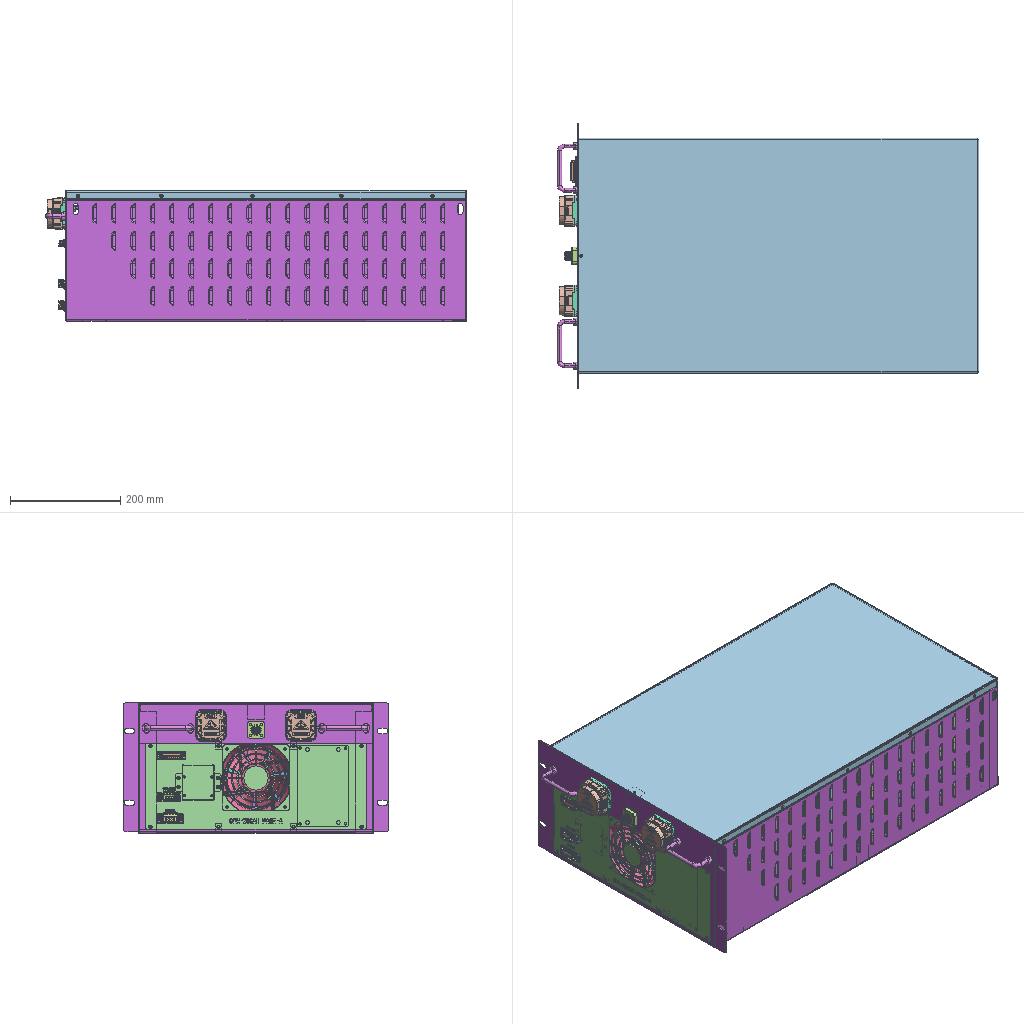Assembly | NX | 135 different items | 178 placed | box 763 x 481 x 237 mm
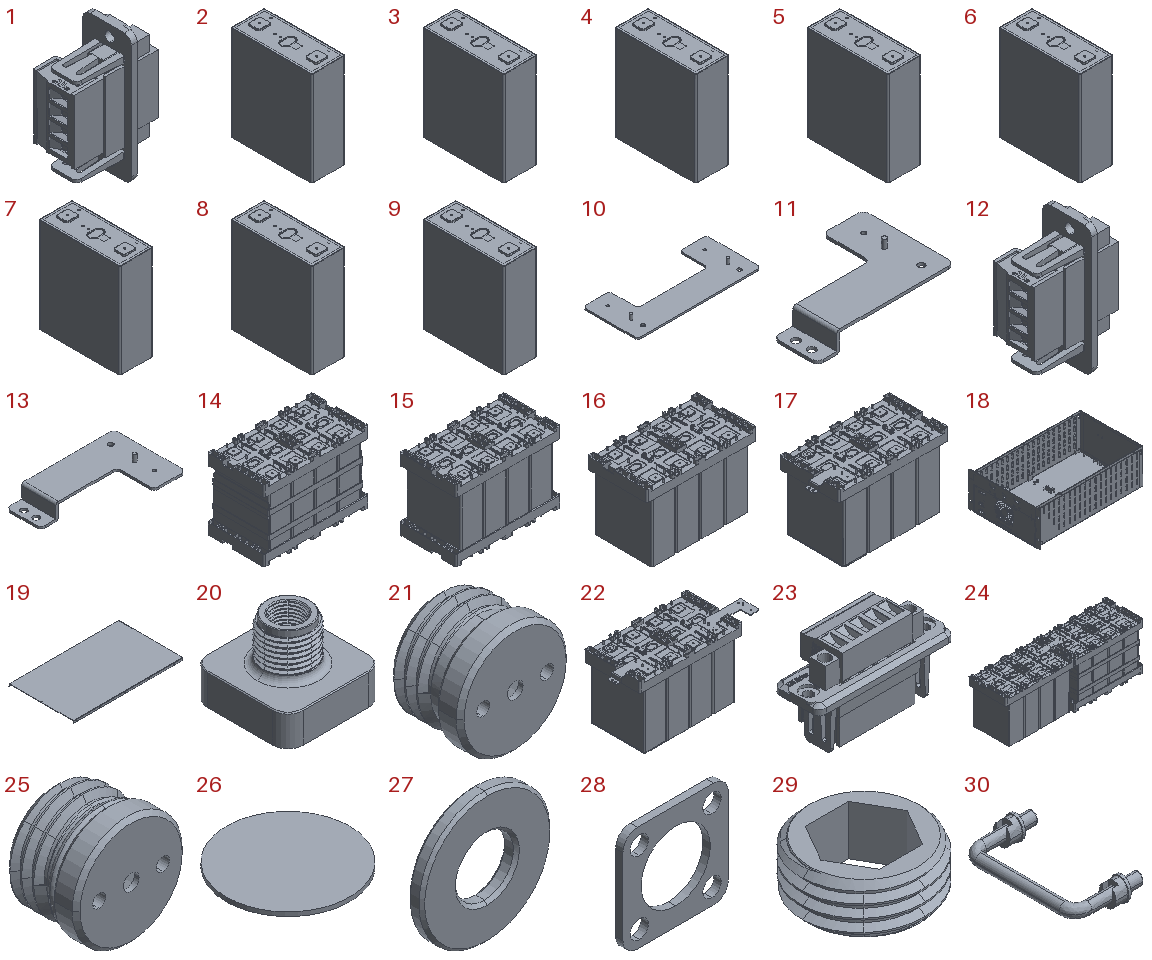Parts list (item | quantity | parent item | size | volume | features):
1 | x1 | - | - | 9257 mm3 | features BREP 21
2 | x1 | in 17 | 71.65 x 173.93 x 207.23 mm | 2540512 mm3 | features BREP 1
3 | x1 | in 16 | 71.65 x 173.93 x 207.23 mm | 2540512 mm3 | features BREP 1
4 | x1 | in 17 | 71.65 x 173.93 x 207.23 mm | 2540512 mm3 | features BREP 1
5 | x1 | in 16 | 71.65 x 173.93 x 207.23 mm | 2540523 mm3 | features BREP 2
6 | x1 | in 17 | 71.65 x 173.93 x 207.23 mm | 2540512 mm3 | features BREP 1
7 | x1 | - | 71.65 x 173.93 x 207.23 mm | 2540512 mm3 | features BREP 1
8 | x1 | - | 71.65 x 173.93 x 207.23 mm | 2540512 mm3 | features BREP 1
9 | x1 | in 14 | 71.65 x 173.93 x 207.23 mm | 2540523 mm3 | features BREP 2
10 | x2 | in 22, 24 | 142 x 62.9 x 8 mm | 12580 mm3 | features BREP 1
11 | x1 | - | 95.45 x 63.5 x 20.5 mm | 8247 mm3 | features BREP 1
12 | x1 | in 70 | - | 9257 mm3 | features BREP 21
13 | x1 | in 17 | 95.45 x 63.5 x 20.5 mm | 8247 mm3 | features BREP 1
14 | x1 | in 24 | 333 x 182 x 228.75 mm | 10791540 mm3 | features BREP 4
15 | x1 | - | 333 x 182 x 227.965 mm | 10643125 mm3 | features BREP 10
16 | x1 | in 24 | 333 x 182 x 217.08 mm | 10398899 mm3 | features BREP 11
17 | x1 | in 22 | 360 x 182 x 216.365 mm | 10554329 mm3 | features BREP 20
18 | x1 | in 38 | - | 1890874 mm3 | features BREP 3
19 | x1 | in 70 | 724.237 x 425.821 x 15 mm | 661919 mm3 | features BREP 1
20 | x1 | in 39 | 31 x 31 x 24 mm | 8742 mm3 | features BREP 1
21 | x1 | in 25 | 13.8 x 9.7 x 13.8 mm | 672.716 mm3 | features BREP 1
22 | x1 | in 94 | 431.925 x 182 x 216.365 mm | 10566909 mm3 | features BREP 21
23 | x1 | - | - | 11022 mm3 | features BREP 24
24 | x1 | in 94 | - | 21203019 mm3 | features BREP 27
25 | x1 | in 39 | 13.8 x 9.7 x 13.8 mm | 702.321 mm3 | features BREP 2
26 | x1 | in 39 | 9 x 9 x 0.3 mm | 19.085 mm3 | features BREP 1
27 | x2 | in 39 | 9 x 1 x 9 mm | 49.417 mm3 | features BREP 1
28 | x1 | in 39 | 29 x 2 x 29 mm | 930.394 mm3 | features BREP 1
29 | x1 | in 39 | 9.9 x 9.9 x 4 mm | 143.224 mm3 | features BREP 1
30 | x2 | in 70 | 51.75 x 94.4 x 18 mm | 11603 mm3 | features BREP 1
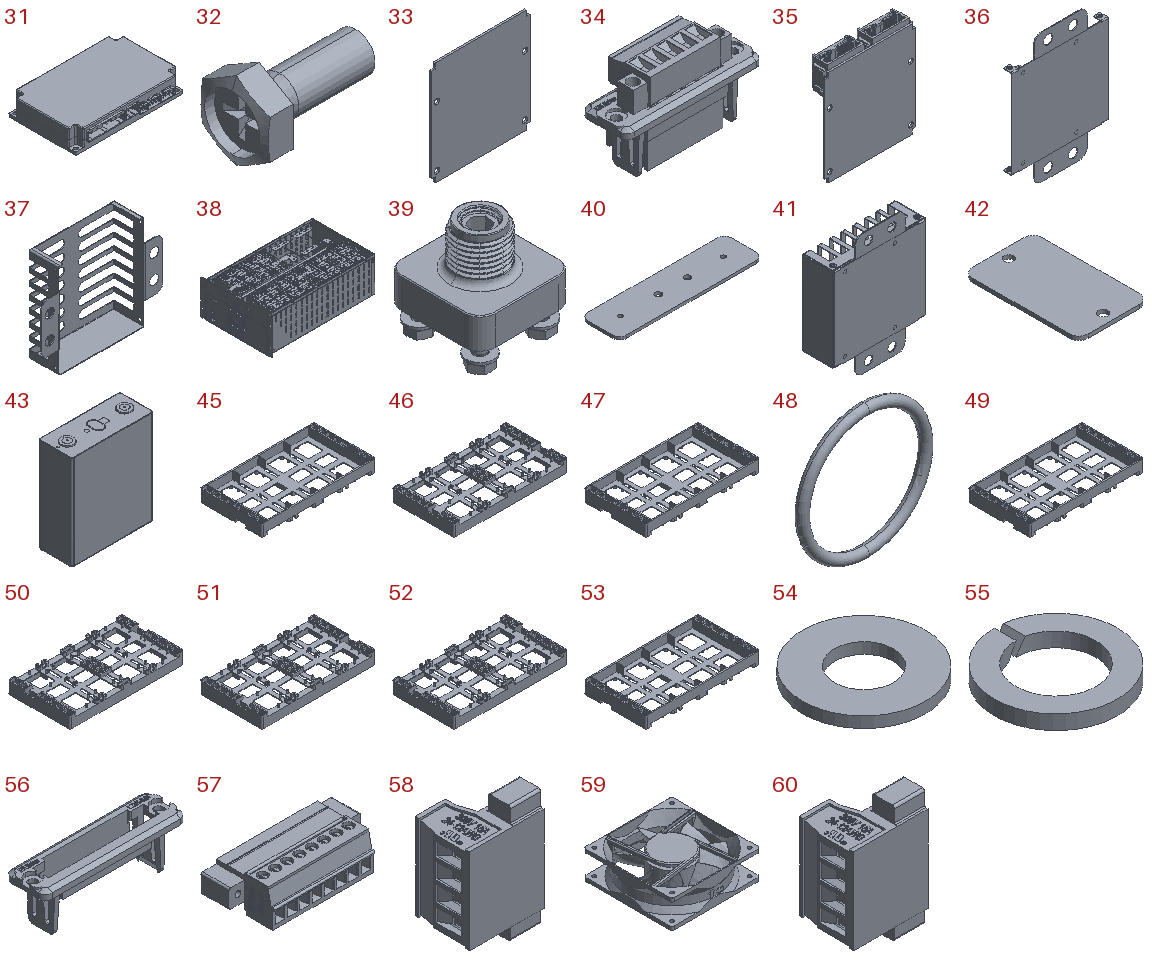31 | x1 | - | 146 x 94 x 27 mm | 100438 mm3 | features BREP 8
32 | x4 | in 74 | 12.8 x 7 x 8.083 mm | 207.191 mm3 | features BREP 1
33 | x1 | in 35 | 56 x 1 x 59 mm | 3252 mm3 | features BREP 1
34 | x1 | in 70 | - | 11022 mm3 | features BREP 24
35 | x1 | in 41 | 56 x 11.171 x 62 mm | 6321 mm3 | features BREP 3
36 | x1 | in 41 | 62.5 x 5.5 x 83 mm | 2275 mm3 | features BREP 1
37 | x1 | in 41 | 82.56 x 21 x 63.94 mm | 2450 mm3 | features BREP 1
38 | x1 | in 70 | - | 33839951 mm3 | features BREP 69
39 | x1 | - | 31 x 31 x 32.5 mm | 11689 mm3 | features BREP 10
40 | x12 | in 94 | 103 x 28 x 8 mm | 5718 mm3 | features BREP 1
41 | x1 | - | 64.47 x 21.5 x 83 mm | 11085 mm3 | features BREP 6
42 | x2 | in 70 | 37 x 61 x 2 mm | 4393 mm3 | features BREP 1
43 | x1 | in 133 | 173.9 x 71.65 x 207.3 mm | 147203 mm3 | features BREP 10
44 | x1 | in 70 | - | - | -
45 | x1 | - | 333 x 182 x 35.5 mm | 236706 mm3 | features BREP 1
46 | x1 | - | 333 x 182 x 35.5 mm | 244246 mm3 | features BREP 1
47 | x1 | - | 333 x 182 x 35.5 mm | 236706 mm3 | features BREP 1
48 | x1 | in 25 | 13 x 1 x 13 mm | 29.609 mm3 | features BREP 1
49 | x1 | - | 333 x 182 x 35.5 mm | 236706 mm3 | features BREP 1
50 | x1 | in 14 | 333 x 182 x 35.5 mm | 236706 mm3 | features BREP 1
51 | x1 | in 17 | 333 x 182 x 35.5 mm | 236706 mm3 | features BREP 1
52 | x1 | in 16 | 333 x 182 x 35.5 mm | 236706 mm3 | features BREP 1
53 | x1 | in 14 | 333 x 182 x 35.5 mm | 236706 mm3 | features BREP 1
54 | x4 | in 74 | 9 x 9 x 0.8 mm | 39.276 mm3 | features BREP 1
55 | x4 | in 74 | 6.8 x 6.8 x 0.8 mm | 16.445 mm3 | features BREP 1
56 | x1 | in 81 | 52.67 x 15 x 18.1 mm | 1861 mm3 | features BREP 1
57 | x1 | in 81 | - | 4072 mm3 | features BREP 19
58 | x1 | in 1 | - | 3758 mm3 | features BREP 11
59 | x1 | in 70 | 119.5 x 119.5 x 38 mm | 147833 mm3 | features BREP 1
60 | x1 | in 12 | - | 3758 mm3 | features BREP 11
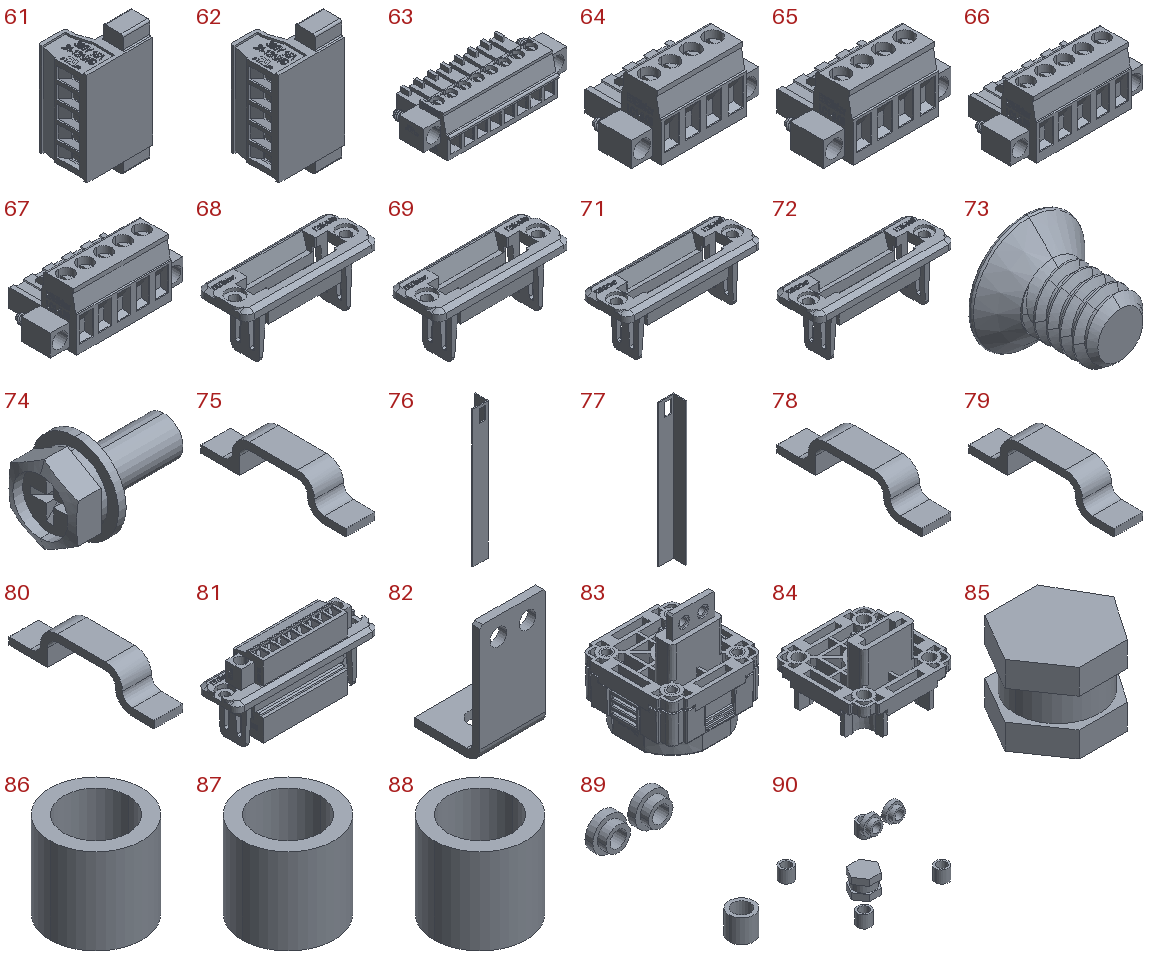61 | x1 | in 23 | - | 4543 mm3 | features BREP 13
62 | x1 | in 34 | - | 4543 mm3 | features BREP 13
63 | x1 | in 81 | 40.98 x 16.1 x 11 mm | 3428 mm3 | features BREP 13
64 | x1 | in 1 | 30.48 x 18.2 x 15 mm | 3734 mm3 | features BREP 9
65 | x1 | in 12 | 30.48 x 18.2 x 15 mm | 3734 mm3 | features BREP 9
66 | x1 | in 23 | 35.56 x 18.2 x 15 mm | 4567 mm3 | features BREP 10
67 | x1 | in 34 | 35.56 x 18.2 x 15 mm | 4567 mm3 | features BREP 10
68 | x1 | in 1 | 44.2 x 16.75 x 19.3 mm | 1766 mm3 | features BREP 1
69 | x1 | in 12 | 44.2 x 16.75 x 19.3 mm | 1766 mm3 | features BREP 1
70 | x1 | - | - | - | features BREP 11
71 | x1 | in 23 | 49.28 x 16.75 x 19.3 mm | 1912 mm3 | features BREP 1
72 | x1 | in 34 | 49.28 x 16.75 x 19.3 mm | 1912 mm3 | features BREP 1
73 | x4 | in 41 | 3.517 x 3 x 3.517 mm | 9.817 mm3 | features BREP 1
74 | x4 | in 39 | 12.8 x 9 x 9 mm | 262.917 mm3 | features BREP 3
75 | x1 | in 94 | 6 x 30 x 7 mm | 342.282 mm3 | features BREP 1
76 | x1 | in 94 | 24.5 x 20.5 x 216 mm | 13794 mm3 | features BREP 1
77 | x1 | in 94 | 24.5 x 20.5 x 216 mm | 13794 mm3 | features BREP 1
78 | x1 | in 94 | 6 x 30 x 7 mm | 342.282 mm3 | features BREP 1
79 | x1 | in 94 | 6 x 30 x 7 mm | 342.282 mm3 | features BREP 1
80 | x1 | in 94 | 6 x 30 x 7 mm | 342.282 mm3 | features BREP 1
81 | x1 | - | - | 9360 mm3 | features BREP 33
82 | x2 | in 93 | 25 x 25 x 45.51 mm | 4597 mm3 | features BREP 1
83 | x2 | in 70 | 56.75 x 56.75 x 64.184 mm | 46396 mm3 | features BREP 10
84 | x2 | in 93 | 56.75 x 56.75 x 38.616 mm | 22776 mm3 | features BREP 1
85 | x2 | in 90 | 13.004 x 11 x 9.5 mm | 595.838 mm3 | features BREP 1
86 | x2 | in 90 | 6.4 x 6.4 x 6 mm | 97.594 mm3 | features BREP 1
87 | x2 | in 90 | 6.4 x 6.4 x 6 mm | 97.594 mm3 | features BREP 1
88 | x2 | in 90 | 6.4 x 6.4 x 6 mm | 97.594 mm3 | features BREP 1
89 | x2 | in 90 | 32.05 x 14.7 x 34.343 mm | 356.162 mm3 | features BREP 3
90 | x2 | in 93 | 44.4 x 44.4 x 39.86 mm | 1245 mm3 | features BREP 7
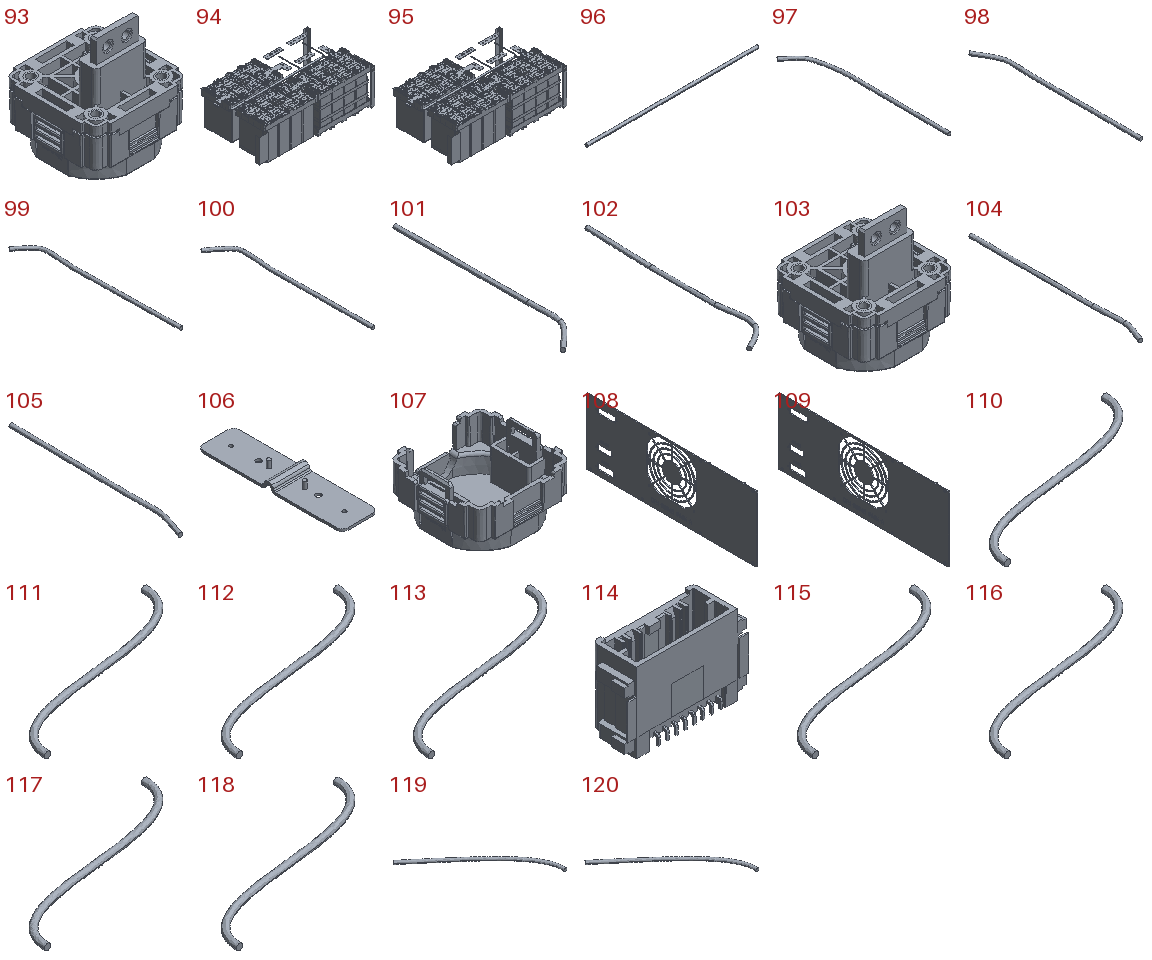91 | x2 | in 93 | - | - | -
92 | x1 | in 70 | - | - | -
93 | x2 | in 103 | 56.75 x 56.75 x 64.184 mm | 46396 mm3 | features BREP 10
94 | x1 | in 95 | - | 31949023 mm3 | features BREP 1
95 | x1 | in 38 | - | 31949023 mm3 | features BREP 65
96 | x1 | in 94 | 581.307 x 10.561 x 10 mm | 45569 mm3 | features BREP 1
97 | x1 | in 94 | 22.885 x 141.616 x 3 mm | 1044 mm3 | features BREP 1
98 | x1 | in 94 | 13.379 x 138.71 x 3 mm | 977.525 mm3 | features BREP 1
99 | x1 | in 94 | 18.288 x 140.353 x 3 mm | 1051 mm3 | features BREP 1
100 | x1 | in 94 | 20.548 x 138.141 x 3 mm | 1002 mm3 | features BREP 1
101 | x1 | in 94 | 20.654 x 142.358 x 3 mm | 1047 mm3 | features BREP 1
102 | x1 | in 94 | 21 x 141.003 x 5.012 mm | 1053 mm3 | features BREP 1
103 | x2 | in 83 | 56.75 x 56.75 x 64.184 mm | 46396 mm3 | features BREP 10
104 | x1 | in 94 | 8.835 x 137.527 x 3 mm | 975.444 mm3 | features BREP 1
105 | x1 | in 94 | 10.731 x 138.267 x 3 mm | 970.254 mm3 | features BREP 1
106 | x1 | in 94 | 30.5 x 121 x 8 mm | 7636 mm3 | features BREP 1
107 | x2 | in 93 | 56.502 x 56.532 x 31.491 mm | 17778 mm3 | features BREP 1
108 | x1 | in 109 | - | - | features BREP 1
109 | x1 | in 18 | - | - | features BREP 1
110 | x1 | in 17 | 31.607 x 15.16 x 1 mm | 29.37 mm3 | features BREP 1
111 | x1 | in 17 | 31.607 x 15.16 x 1 mm | 29.37 mm3 | features BREP 1
112 | x1 | - | 31.607 x 15.16 x 1 mm | 29.37 mm3 | features BREP 1
113 | x1 | - | 31.607 x 15.16 x 1 mm | 29.37 mm3 | features BREP 1
114 | x1 | in 35 | 27.19 x 10.174 x 17.8 mm | 1535 mm3 | features BREP 1
115 | x1 | in 16 | 31.607 x 15.16 x 1 mm | 29.37 mm3 | features BREP 1
116 | x1 | in 14 | 31.607 x 15.16 x 1 mm | 29.37 mm3 | features BREP 1
117 | x1 | in 14 | 31.607 x 15.16 x 1 mm | 29.37 mm3 | features BREP 1
118 | x1 | in 16 | 31.607 x 15.16 x 1 mm | 29.37 mm3 | features BREP 1
119 | x1 | in 17 | 26.795 x 30.33 x 1.202 mm | 31.795 mm3 | features BREP 1
120 | x1 | in 17 | 26.795 x 30.33 x 1.202 mm | 31.795 mm3 | features BREP 1
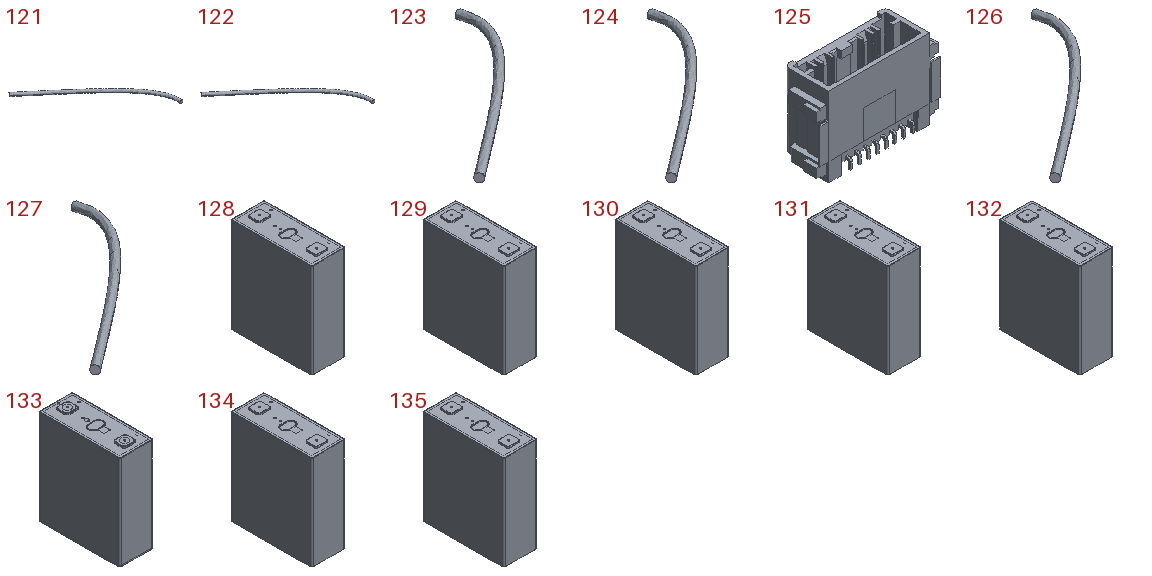121 | x1 | - | 26.795 x 30.33 x 1.202 mm | 31.795 mm3 | features BREP 1
122 | x1 | - | 26.795 x 30.33 x 1.202 mm | 31.795 mm3 | features BREP 1
123 | x1 | in 16 | 26.795 x 29.055 x 10.011 mm | 31.795 mm3 | features BREP 1
124 | x1 | in 14 | 26.795 x 29.055 x 10.011 mm | 31.795 mm3 | features BREP 1
125 | x1 | in 35 | 27.19 x 10.174 x 17.8 mm | 1535 mm3 | features BREP 1
126 | x1 | in 14 | 26.795 x 29.055 x 10.011 mm | 31.795 mm3 | features BREP 1
127 | x1 | in 16 | 26.795 x 29.055 x 10.011 mm | 31.795 mm3 | features BREP 1
128 | x1 | in 14 | 71.65 x 173.93 x 207.23 mm | 2540512 mm3 | features BREP 1
129 | x1 | in 14 | 71.65 x 173.93 x 207.23 mm | 2540512 mm3 | features BREP 1
130 | x1 | in 16 | 71.65 x 173.93 x 207.23 mm | 2540512 mm3 | features BREP 1
131 | x1 | in 14 | 71.65 x 173.93 x 207.23 mm | 2540512 mm3 | features BREP 1
132 | x1 | - | 71.65 x 173.93 x 207.23 mm | 2540512 mm3 | features BREP 1
133 | x1 | in 17 | 71.65 x 173.97 x 207.3 mm | 2687716 mm3 | features BREP 1
134 | x1 | in 16 | 71.65 x 173.93 x 207.23 mm | 2540523 mm3 | features BREP 2
135 | x1 | - | 71.65 x 173.93 x 207.23 mm | 2540512 mm3 | features BREP 1